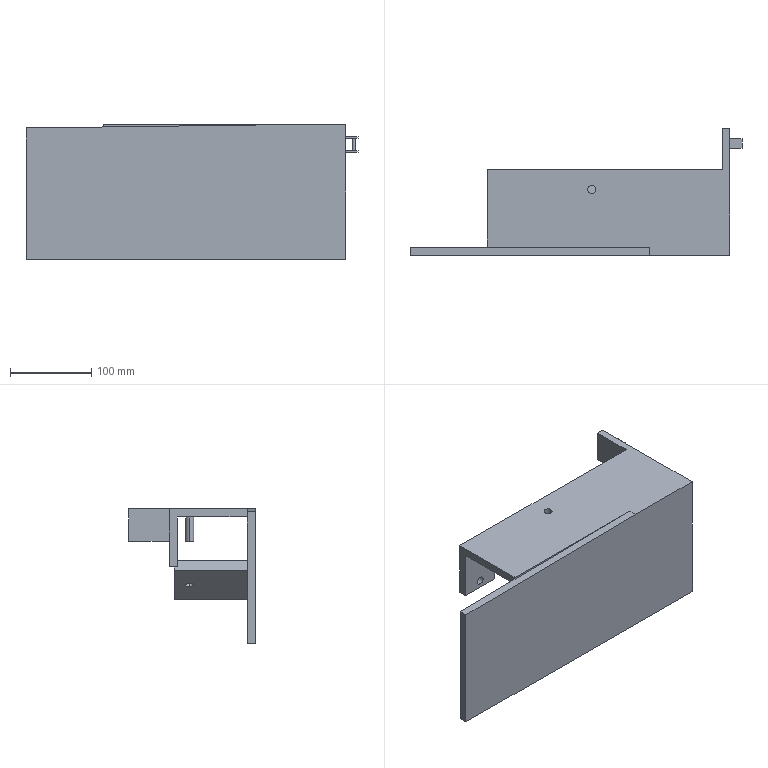Part | SolidWorks | features ICE 36, Extrusion 1, Sweep 1 | 1 solid | 46 faces | box 408.883 x 156 x 165.33 mm | volume 1077828 mm3 | plane 36 | cylinder 10 | commonest cylinder face diameters 10 x8 4 x2
STEP:
#1=CARTESIAN_POINT('',(-112.206,25.,-64.041));
#2=VERTEX_POINT('',#1);
#3=CARTESIAN_POINT('',(-121.034,25.,-59.342));
#4=VERTEX_POINT('',#3);
#5=CARTESIAN_POINT('',(-116.62,25.,-61.691));
#6=DIRECTION('',(-0.4698,0.,-0.8827));
#7=DIRECTION('',(-0.8827,0.,0.4698));
#8=AXIS2_PLACEMENT_3D('',#5,#6,#7);
#9=CIRCLE('',#8,5.);
#10=EDGE_CURVE('',#2,#4,#9,.T.);
#11=ORIENTED_EDGE('',*,*,#10,.F.);
#12=CARTESIAN_POINT('',(-118.59,25.,-76.034));
#13=VERTEX_POINT('',#12);
#14=CARTESIAN_POINT('',(-104.494,25.,-49.551));
#15=DIRECTION('',(-0.4698,0.,-0.8827));
#16=VECTOR('',#15,1000.);
#17=LINE('',#14,#16);
#18=EDGE_CURVE('',#2,#13,#17,.T.);
#19=ORIENTED_EDGE('',*,*,#18,.T.);
#20=CARTESIAN_POINT('',(-127.417,25.,-71.335));
#21=VERTEX_POINT('',#20);
#22=CARTESIAN_POINT('',(-123.003,25.,-73.685));
#23=DIRECTION('',(-0.4698,0.,-0.8827));
#24=DIRECTION('',(-0.8827,0.,0.4698));
#25=AXIS2_PLACEMENT_3D('',#22,#23,#24);
#26=CIRCLE('',#25,5.);
#27=EDGE_CURVE('',#13,#21,#26,.T.);
#28=ORIENTED_EDGE('',*,*,#27,.T.);
#29=CARTESIAN_POINT('',(-113.322,25.,-44.853));
#30=DIRECTION('',(-0.4698,0.,-0.8827));
#31=VECTOR('',#30,1000.);
#32=LINE('',#29,#31);
#33=EDGE_CURVE('',#4,#21,#32,.T.);
#34=ORIENTED_EDGE('',*,*,#33,.F.);
#35=EDGE_LOOP('',(#11,#19,#28,#34));
#36=FACE_OUTER_BOUND('',#35,.T.);
#37=CARTESIAN_POINT('',(-108.908,25.,-47.202));
#38=DIRECTION('',(-0.4698,0.,-0.8827));
#39=DIRECTION('',(-0.8827,0.,0.4698));
#40=AXIS2_PLACEMENT_3D('',#37,#38,#39);
#41=CYLINDRICAL_SURFACE('',#40,5.);
#42=ADVANCED_FACE('',(#36),#41,.F.);
#43=CARTESIAN_POINT('',(-209.637,40.,-45.397));
#44=VERTEX_POINT('',#43);
#45=CARTESIAN_POINT('',(-209.637,40.,-35.397));
#46=VERTEX_POINT('',#45);
#47=CARTESIAN_POINT('',(-209.637,40.,-40.397));
#48=DIRECTION('',(0.,1.,0.));
#49=DIRECTION('',(0.,0.,1.));
#50=AXIS2_PLACEMENT_3D('',#47,#48,#49);
#51=CIRCLE('',#50,5.);
#52=EDGE_CURVE('',#44,#46,#51,.T.);
#53=ORIENTED_EDGE('',*,*,#52,.F.);
#54=CARTESIAN_POINT('',(-209.637,50.,-45.397));
#55=VERTEX_POINT('',#54);
#56=CARTESIAN_POINT('',(-209.637,40.,-45.397));
#57=DIRECTION('',(0.,1.,0.));
#58=VECTOR('',#57,1000.);
#59=LINE('',#56,#58);
#60=EDGE_CURVE('',#44,#55,#59,.T.);
#61=ORIENTED_EDGE('',*,*,#60,.T.);
#62=CARTESIAN_POINT('',(-209.637,50.,-35.397));
#63=VERTEX_POINT('',#62);
#64=CARTESIAN_POINT('',(-209.637,50.,-40.397));
#65=DIRECTION('',(0.,1.,0.));
#66=DIRECTION('',(0.,0.,1.));
#67=AXIS2_PLACEMENT_3D('',#64,#65,#66);
#68=CIRCLE('',#67,5.);
#69=EDGE_CURVE('',#55,#63,#68,.T.);
#70=ORIENTED_EDGE('',*,*,#69,.T.);
#71=CARTESIAN_POINT('',(-209.637,40.,-35.397));
#72=DIRECTION('',(0.,1.,0.));
#73=VECTOR('',#72,1000.);
#74=LINE('',#71,#73);
#75=EDGE_CURVE('',#46,#63,#74,.T.);
#76=ORIENTED_EDGE('',*,*,#75,.F.);
#77=EDGE_LOOP('',(#53,#61,#70,#76));
#78=FACE_OUTER_BOUND('',#77,.T.);
#79=CARTESIAN_POINT('',(-209.637,40.,-40.397));
#80=DIRECTION('',(0.,1.,0.));
#81=DIRECTION('',(0.,0.,1.));
#82=AXIS2_PLACEMENT_3D('',#79,#80,#81);
#83=CYLINDRICAL_SURFACE('',#82,5.);
#84=ADVANCED_FACE('',(#78),#83,.F.);
#85=CARTESIAN_POINT('',(-101.44,25.,20.176));
#86=VERTEX_POINT('',#85);
#87=CARTESIAN_POINT('',(-111.44,25.,20.176));
#88=VERTEX_POINT('',#87);
#89=CARTESIAN_POINT('',(-106.44,25.,20.176));
#90=DIRECTION('',(0.,0.,-1.));
#91=DIRECTION('',(-1.,0.,0.));
#92=AXIS2_PLACEMENT_3D('',#89,#90,#91);
#93=CIRCLE('',#92,5.);
#94=EDGE_CURVE('',#86,#88,#93,.T.);
#95=ORIENTED_EDGE('',*,*,#94,.F.);
#96=CARTESIAN_POINT('',(-101.44,25.,10.176));
#97=VERTEX_POINT('',#96);
#98=CARTESIAN_POINT('',(-101.44,25.,210.176));
#99=DIRECTION('',(0.,0.,-1.));
#100=VECTOR('',#99,1000.);
#101=LINE('',#98,#100);
#102=EDGE_CURVE('',#86,#97,#101,.T.);
#103=ORIENTED_EDGE('',*,*,#102,.T.);
#104=CARTESIAN_POINT('',(-111.44,25.,10.176));
#105=VERTEX_POINT('',#104);
#106=CARTESIAN_POINT('',(-106.44,25.,10.176));
#107=DIRECTION('',(0.,0.,-1.));
#108=DIRECTION('',(-1.,0.,0.));
#109=AXIS2_PLACEMENT_3D('',#106,#107,#108);
#110=CIRCLE('',#109,5.);
#111=EDGE_CURVE('',#97,#105,#110,.T.);
#112=ORIENTED_EDGE('',*,*,#111,.T.);
#113=CARTESIAN_POINT('',(-111.44,25.,210.176));
#114=DIRECTION('',(0.,0.,-1.));
#115=VECTOR('',#114,1000.);
#116=LINE('',#113,#115);
#117=EDGE_CURVE('',#88,#105,#116,.T.);
#118=ORIENTED_EDGE('',*,*,#117,.F.);
#119=EDGE_LOOP('',(#95,#103,#112,#118));
#120=FACE_OUTER_BOUND('',#119,.T.);
#121=CARTESIAN_POINT('',(-106.44,25.,210.176));
#122=DIRECTION('',(0.,0.,-1.));
#123=DIRECTION('',(-1.,0.,0.));
#124=AXIS2_PLACEMENT_3D('',#121,#122,#123);
#125=CYLINDRICAL_SURFACE('',#124,5.);
#126=ADVANCED_FACE('',(#120),#125,.F.);
#127=CARTESIAN_POINT('',(71.457,81.541,-11.824));
#128=VERTEX_POINT('',#127);
#129=CARTESIAN_POINT('',(75.457,81.541,-11.824));
#130=VERTEX_POINT('',#129);
#131=CARTESIAN_POINT('',(73.457,81.541,-11.824));
#132=DIRECTION('',(0.,0.,-1.));
#133=DIRECTION('',(-1.,0.,0.));
#134=AXIS2_PLACEMENT_3D('',#131,#132,#133);
#135=CIRCLE('',#134,2.);
#136=EDGE_CURVE('',#128,#130,#135,.T.);
#137=ORIENTED_EDGE('',*,*,#136,.F.);
#138=CARTESIAN_POINT('',(71.457,81.541,3.56));
#139=VERTEX_POINT('',#138);
#140=CARTESIAN_POINT('',(71.457,81.541,-12.44));
#141=DIRECTION('',(0.,0.,1.));
#142=VECTOR('',#141,1000.);
#143=LINE('',#140,#142);
#144=EDGE_CURVE('',#128,#139,#143,.T.);
#145=ORIENTED_EDGE('',*,*,#144,.T.);
#146=CARTESIAN_POINT('',(75.457,81.541,3.56));
#147=VERTEX_POINT('',#146);
#148=CARTESIAN_POINT('',(73.457,81.541,3.56));
#149=DIRECTION('',(0.,0.,1.));
#150=DIRECTION('',(1.,0.,0.));
#151=AXIS2_PLACEMENT_3D('',#148,#149,#150);
#152=CIRCLE('',#151,2.);
#153=EDGE_CURVE('',#147,#139,#152,.T.);
#154=ORIENTED_EDGE('',*,*,#153,.F.);
#155=CARTESIAN_POINT('',(75.457,81.541,-12.44));
#156=DIRECTION('',(0.,0.,1.));
#157=VECTOR('',#156,1000.);
#158=LINE('',#155,#157);
#159=EDGE_CURVE('',#130,#147,#158,.T.);
#160=ORIENTED_EDGE('',*,*,#159,.F.);
#161=EDGE_LOOP('',(#137,#145,#154,#160));
#162=FACE_OUTER_BOUND('',#161,.T.);
#163=CARTESIAN_POINT('',(73.457,81.541,-12.44));
#164=DIRECTION('',(0.,0.,1.));
#165=DIRECTION('',(1.,0.,0.));
#166=AXIS2_PLACEMENT_3D('',#163,#164,#165);
#167=CYLINDRICAL_SURFACE('',#166,2.);
#168=ADVANCED_FACE('',(#162),#167,.T.);
#169=CARTESIAN_POINT('',(-21.44,25.,-19.824));
#170=VERTEX_POINT('',#169);
#171=CARTESIAN_POINT('',(-11.44,25.,-19.824));
#172=VERTEX_POINT('',#171);
#173=CARTESIAN_POINT('',(-16.44,25.,-19.824));
#174=DIRECTION('',(0.,0.,-1.));
#175=DIRECTION('',(1.,0.,0.));
#176=AXIS2_PLACEMENT_3D('',#173,#174,#175);
#177=CIRCLE('',#176,5.);
#178=EDGE_CURVE('',#170,#172,#177,.T.);
#179=ORIENTED_EDGE('',*,*,#178,.F.);
#180=CARTESIAN_POINT('',(-21.44,25.,10.176));
#181=VERTEX_POINT('',#180);
#182=CARTESIAN_POINT('',(-21.44,25.,-33.966));
#183=DIRECTION('',(0.,0.,1.));
#184=VECTOR('',#183,1000.);
#185=LINE('',#182,#184);
#186=EDGE_CURVE('',#170,#181,#185,.T.);
#187=ORIENTED_EDGE('',*,*,#186,.T.);
#188=CARTESIAN_POINT('',(-11.44,25.,10.176));
#189=VERTEX_POINT('',#188);
#190=CARTESIAN_POINT('',(-16.44,25.,10.176));
#191=DIRECTION('',(0.,0.,-1.));
#192=DIRECTION('',(1.,0.,0.));
#193=AXIS2_PLACEMENT_3D('',#190,#191,#192);
#194=CIRCLE('',#193,5.);
#195=EDGE_CURVE('',#181,#189,#194,.T.);
#196=ORIENTED_EDGE('',*,*,#195,.T.);
#197=CARTESIAN_POINT('',(-11.44,25.,-33.966));
#198=DIRECTION('',(0.,0.,1.));
#199=VECTOR('',#198,1000.);
#200=LINE('',#197,#199);
#201=EDGE_CURVE('',#172,#189,#200,.T.);
#202=ORIENTED_EDGE('',*,*,#201,.F.);
#203=EDGE_LOOP('',(#179,#187,#196,#202));
#204=FACE_OUTER_BOUND('',#203,.T.);
#205=CARTESIAN_POINT('',(-16.44,25.,-33.966));
#206=DIRECTION('',(0.,0.,1.));
#207=DIRECTION('',(1.,0.,0.));
#208=AXIS2_PLACEMENT_3D('',#205,#206,#207);
#209=CYLINDRICAL_SURFACE('',#208,5.);
#210=ADVANCED_FACE('',(#204),#209,.T.);
#211=CARTESIAN_POINT('',(63.457,-46.,10.176));
#212=VERTEX_POINT('',#211);
#213=CARTESIAN_POINT('',(63.457,-46.,-145.154));
#214=VERTEX_POINT('',#213);
#215=CARTESIAN_POINT('',(63.457,-46.,20.176));
#216=DIRECTION('',(0.,0.,-1.));
#217=VECTOR('',#216,1000.);
#218=LINE('',#215,#217);
#219=EDGE_CURVE('',#212,#214,#218,.T.);
#220=ORIENTED_EDGE('',*,*,#219,.T.);
#221=CARTESIAN_POINT('',(-330.425,-46.,-145.154));
#222=VERTEX_POINT('',#221);
#223=CARTESIAN_POINT('',(-330.425,-46.,-145.154));
#224=DIRECTION('',(1.,0.,0.));
#225=VECTOR('',#224,1000.);
#226=LINE('',#223,#225);
#227=EDGE_CURVE('',#222,#214,#226,.T.);
#228=ORIENTED_EDGE('',*,*,#227,.F.);
#229=CARTESIAN_POINT('',(-330.425,-46.,16.345));
#230=VERTEX_POINT('',#229);
#231=CARTESIAN_POINT('',(-330.425,-46.,-189.172));
#232=DIRECTION('',(0.,0.,-1.));
#233=VECTOR('',#232,1000.);
#234=LINE('',#231,#233);
#235=EDGE_CURVE('',#230,#222,#234,.T.);
#236=ORIENTED_EDGE('',*,*,#235,.F.);
#237=CARTESIAN_POINT('',(-235.023,-46.,17.582));
#238=VERTEX_POINT('',#237);
#239=CARTESIAN_POINT('',(-35.023,-46.,20.176));
#240=DIRECTION('',(0.9999,0.,0.01297));
#241=VECTOR('',#240,1000.);
#242=LINE('',#239,#241);
#243=EDGE_CURVE('',#230,#238,#242,.T.);
#244=ORIENTED_EDGE('',*,*,#243,.T.);
#245=CARTESIAN_POINT('',(-235.023,-46.,10.176));
#246=VERTEX_POINT('',#245);
#247=CARTESIAN_POINT('',(-235.023,-46.,10.176));
#248=DIRECTION('',(0.,0.,1.));
#249=VECTOR('',#248,1000.);
#250=LINE('',#247,#249);
#251=EDGE_CURVE('',#246,#238,#250,.T.);
#252=ORIENTED_EDGE('',*,*,#251,.F.);
#253=CARTESIAN_POINT('',(-35.023,-46.,10.176));
#254=DIRECTION('',(-1.,0.,0.));
#255=VECTOR('',#254,1000.);
#256=LINE('',#253,#255);
#257=EDGE_CURVE('',#212,#246,#256,.T.);
#258=ORIENTED_EDGE('',*,*,#257,.F.);
#259=EDGE_LOOP('',(#220,#228,#236,#244,#252,#258));
#260=FACE_OUTER_BOUND('',#259,.T.);
#261=CARTESIAN_POINT('',(-88.62,-46.,-91.985));
#262=VERTEX_POINT('',#261);
#263=CARTESIAN_POINT('',(-157.387,-46.,-55.384));
#264=VERTEX_POINT('',#263);
#265=CARTESIAN_POINT('',(-100.648,-46.,-85.583));
#266=DIRECTION('',(-0.8827,0.,0.4698));
#267=VECTOR('',#266,1000.);
#268=LINE('',#265,#267);
#269=EDGE_CURVE('',#262,#264,#268,.T.);
#270=ORIENTED_EDGE('',*,*,#269,.F.);
#271=CARTESIAN_POINT('',(-82.236,-46.,-79.992));
#272=VERTEX_POINT('',#271);
#273=CARTESIAN_POINT('',(-88.62,-46.,-91.985));
#274=DIRECTION('',(-0.4698,0.,-0.8827));
#275=VECTOR('',#274,1000.);
#276=LINE('',#273,#275);
#277=EDGE_CURVE('',#272,#262,#276,.T.);
#278=ORIENTED_EDGE('',*,*,#277,.F.);
#279=CARTESIAN_POINT('',(-151.003,-46.,-43.391));
#280=VERTEX_POINT('',#279);
#281=CARTESIAN_POINT('',(-82.236,-46.,-79.992));
#282=DIRECTION('',(0.8827,0.,-0.4698));
#283=VECTOR('',#282,1000.);
#284=LINE('',#281,#283);
#285=EDGE_CURVE('',#280,#272,#284,.T.);
#286=ORIENTED_EDGE('',*,*,#285,.F.);
#287=CARTESIAN_POINT('',(-157.387,-46.,-55.384));
#288=DIRECTION('',(0.4698,0.,0.8827));
#289=VECTOR('',#288,1000.);
#290=LINE('',#287,#289);
#291=EDGE_CURVE('',#264,#280,#290,.T.);
#292=ORIENTED_EDGE('',*,*,#291,.F.);
#293=EDGE_LOOP('',(#270,#278,#286,#292));
#294=FACE_BOUND('',#293,.T.);
#295=CARTESIAN_POINT('',(0.,-46.,0.));
#296=DIRECTION('',(0.,-1.,0.));
#297=DIRECTION('',(0.,0.,-1.));
#298=AXIS2_PLACEMENT_3D('',#295,#296,#297);
#299=PLANE('',#298);
#300=ADVANCED_FACE('',(#260,#294),#299,.F.);
#301=CARTESIAN_POINT('',(-209.637,50.,-40.397));
#302=DIRECTION('',(0.,1.,0.));
#303=DIRECTION('',(0.,0.,1.));
#304=AXIS2_PLACEMENT_3D('',#301,#302,#303);
#305=CIRCLE('',#304,5.);
#306=EDGE_CURVE('',#63,#55,#305,.T.);
#307=ORIENTED_EDGE('',*,*,#306,.F.);
#308=ORIENTED_EDGE('',*,*,#69,.F.);
#309=EDGE_LOOP('',(#307,#308));
#310=FACE_BOUND('',#309,.T.);
#311=CARTESIAN_POINT('',(-184.251,50.,10.176));
#312=VERTEX_POINT('',#311);
#313=CARTESIAN_POINT('',(54.56,50.,10.176));
#314=VERTEX_POINT('',#313);
#315=CARTESIAN_POINT('',(-161.43,50.,10.176));
#316=DIRECTION('',(1.,0.,0.));
#317=VECTOR('',#316,1000.);
#318=LINE('',#315,#317);
#319=EDGE_CURVE('',#312,#314,#318,.T.);
#320=ORIENTED_EDGE('',*,*,#319,.F.);
#321=CARTESIAN_POINT('',(-184.251,50.,-50.397));
#322=VERTEX_POINT('',#321);
#323=CARTESIAN_POINT('',(-184.251,50.,10.176));
#324=DIRECTION('',(0.,0.,-1.));
#325=VECTOR('',#324,1000.);
#326=LINE('',#323,#325);
#327=EDGE_CURVE('',#312,#322,#326,.T.);
#328=ORIENTED_EDGE('',*,*,#327,.T.);
#329=CARTESIAN_POINT('',(-235.023,50.,-50.397));
#330=VERTEX_POINT('',#329);
#331=CARTESIAN_POINT('',(-235.023,50.,-50.397));
#332=DIRECTION('',(-1.,0.,0.));
#333=VECTOR('',#332,1000.);
#334=LINE('',#331,#333);
#335=EDGE_CURVE('',#322,#330,#334,.T.);
#336=ORIENTED_EDGE('',*,*,#335,.T.);
#337=CARTESIAN_POINT('',(-235.023,50.,20.176));
#338=VERTEX_POINT('',#337);
#339=CARTESIAN_POINT('',(-235.023,50.,10.176));
#340=DIRECTION('',(0.,0.,-1.));
#341=VECTOR('',#340,1000.);
#342=LINE('',#339,#341);
#343=EDGE_CURVE('',#338,#330,#342,.T.);
#344=ORIENTED_EDGE('',*,*,#343,.F.);
#345=CARTESIAN_POINT('',(54.56,50.,20.176));
#346=VERTEX_POINT('',#345);
#347=CARTESIAN_POINT('',(-110.44,50.,20.176));
#348=DIRECTION('',(-1.,0.,0.));
#349=VECTOR('',#348,1000.);
#350=LINE('',#347,#349);
#351=EDGE_CURVE('',#346,#338,#350,.T.);
#352=ORIENTED_EDGE('',*,*,#351,.F.);
#353=CARTESIAN_POINT('',(54.56,50.,20.176));
#354=DIRECTION('',(0.,0.,-1.));
#355=VECTOR('',#354,1000.);
#356=LINE('',#353,#355);
#357=EDGE_CURVE('',#346,#314,#356,.T.);
#358=ORIENTED_EDGE('',*,*,#357,.T.);
#359=EDGE_LOOP('',(#320,#328,#336,#344,#352,#358));
#360=FACE_OUTER_BOUND('',#359,.T.);
#361=CARTESIAN_POINT('',(0.,50.,0.));
#362=DIRECTION('',(0.,-1.,0.));
#363=DIRECTION('',(0.,0.,-1.));
#364=AXIS2_PLACEMENT_3D('',#361,#362,#363);
#365=PLANE('',#364);
#366=ADVANCED_FACE('',(#310,#360),#365,.F.);
#367=CARTESIAN_POINT('',(-106.44,25.,20.176));
#368=DIRECTION('',(0.,0.,-1.));
#369=DIRECTION('',(-1.,0.,0.));
#370=AXIS2_PLACEMENT_3D('',#367,#368,#369);
#371=CIRCLE('',#370,5.);
#372=EDGE_CURVE('',#88,#86,#371,.T.);
#373=ORIENTED_EDGE('',*,*,#372,.T.);
#374=ORIENTED_EDGE('',*,*,#94,.T.);
#375=EDGE_LOOP('',(#373,#374));
#376=FACE_BOUND('',#375,.T.);
#377=ORIENTED_EDGE('',*,*,#351,.T.);
#378=CARTESIAN_POINT('',(-235.023,-46.,20.176));
#379=VERTEX_POINT('',#378);
#380=CARTESIAN_POINT('',(-235.023,50.,20.176));
#381=DIRECTION('',(0.,1.,0.));
#382=VECTOR('',#381,1000.);
#383=LINE('',#380,#382);
#384=EDGE_CURVE('',#379,#338,#383,.T.);
#385=ORIENTED_EDGE('',*,*,#384,.F.);
#386=CARTESIAN_POINT('',(-35.023,-46.,20.176));
#387=VERTEX_POINT('',#386);
#388=CARTESIAN_POINT('',(-235.023,-46.,20.176));
#389=DIRECTION('',(1.,0.,0.));
#390=VECTOR('',#389,1000.);
#391=LINE('',#388,#390);
#392=EDGE_CURVE('',#379,#387,#391,.T.);
#393=ORIENTED_EDGE('',*,*,#392,.T.);
#394=CARTESIAN_POINT('',(-35.023,-56.,20.176));
#395=VERTEX_POINT('',#394);
#396=CARTESIAN_POINT('',(-35.023,-46.,20.176));
#397=DIRECTION('',(0.,-1.,0.));
#398=VECTOR('',#397,1000.);
#399=LINE('',#396,#398);
#400=EDGE_CURVE('',#387,#395,#399,.T.);
#401=ORIENTED_EDGE('',*,*,#400,.T.);
#402=CARTESIAN_POINT('',(63.457,-56.,20.176));
#403=VERTEX_POINT('',#402);
#404=CARTESIAN_POINT('',(-35.023,-56.,20.176));
#405=DIRECTION('',(1.,0.,0.));
#406=VECTOR('',#405,1000.);
#407=LINE('',#404,#406);
#408=EDGE_CURVE('',#395,#403,#407,.T.);
#409=ORIENTED_EDGE('',*,*,#408,.T.);
#410=CARTESIAN_POINT('',(63.457,100.,20.176));
#411=VERTEX_POINT('',#410);
#412=CARTESIAN_POINT('',(63.457,-0.000025,20.176));
#413=DIRECTION('',(0.,1.,0.));
#414=VECTOR('',#413,1000.);
#415=LINE('',#412,#414);
#416=EDGE_CURVE('',#403,#411,#415,.T.);
#417=ORIENTED_EDGE('',*,*,#416,.T.);
#418=CARTESIAN_POINT('',(54.56,100.,20.176));
#419=VERTEX_POINT('',#418);
#420=CARTESIAN_POINT('',(54.56,100.,20.176));
#421=DIRECTION('',(-1.,0.,0.));
#422=VECTOR('',#421,1000.);
#423=LINE('',#420,#422);
#424=EDGE_CURVE('',#411,#419,#423,.T.);
#425=ORIENTED_EDGE('',*,*,#424,.T.);
#426=CARTESIAN_POINT('',(54.56,100.,20.176));
#427=DIRECTION('',(0.,-1.,0.));
#428=VECTOR('',#427,1000.);
#429=LINE('',#426,#428);
#430=EDGE_CURVE('',#419,#346,#429,.T.);
#431=ORIENTED_EDGE('',*,*,#430,.T.);
#432=EDGE_LOOP('',(#377,#385,#393,#401,#409,#417,#425,#431));
#433=FACE_OUTER_BOUND('',#432,.T.);
#434=CARTESIAN_POINT('',(0.,0.,20.176));
#435=DIRECTION('',(0.,0.,-1.));
#436=DIRECTION('',(-1.,0.,0.));
#437=AXIS2_PLACEMENT_3D('',#434,#435,#436);
#438=PLANE('',#437);
#439=ADVANCED_FACE('',(#376,#433),#438,.F.);
#440=CARTESIAN_POINT('',(-106.44,25.,10.176));
#441=DIRECTION('',(0.,0.,-1.));
#442=DIRECTION('',(-1.,0.,0.));
#443=AXIS2_PLACEMENT_3D('',#440,#441,#442);
#444=CIRCLE('',#443,5.);
#445=EDGE_CURVE('',#105,#97,#444,.T.);
#446=ORIENTED_EDGE('',*,*,#445,.F.);
#447=ORIENTED_EDGE('',*,*,#111,.F.);
#448=EDGE_LOOP('',(#446,#447));
#449=FACE_BOUND('',#448,.T.);
#450=CARTESIAN_POINT('',(-16.44,25.,10.176));
#451=DIRECTION('',(0.,0.,-1.));
#452=DIRECTION('',(1.,0.,0.));
#453=AXIS2_PLACEMENT_3D('',#450,#451,#452);
#454=CIRCLE('',#453,5.);
#455=EDGE_CURVE('',#189,#181,#454,.T.);
#456=ORIENTED_EDGE('',*,*,#455,.F.);
#457=ORIENTED_EDGE('',*,*,#195,.F.);
#458=EDGE_LOOP('',(#456,#457));
#459=FACE_BOUND('',#458,.T.);
#460=CARTESIAN_POINT('',(-235.023,40.,10.176));
#461=VERTEX_POINT('',#460);
#462=CARTESIAN_POINT('',(-184.251,40.,10.176));
#463=VERTEX_POINT('',#462);
#464=CARTESIAN_POINT('',(-235.023,40.,10.176));
#465=DIRECTION('',(1.,0.,0.));
#466=VECTOR('',#465,1000.);
#467=LINE('',#464,#466);
#468=EDGE_CURVE('',#461,#463,#467,.T.);
#469=ORIENTED_EDGE('',*,*,#468,.T.);
#470=CARTESIAN_POINT('',(-184.251,40.,10.176));
#471=DIRECTION('',(0.,1.,0.));
#472=VECTOR('',#471,1000.);
#473=LINE('',#470,#472);
#474=EDGE_CURVE('',#463,#312,#473,.T.);
#475=ORIENTED_EDGE('',*,*,#474,.T.);
#476=ORIENTED_EDGE('',*,*,#319,.T.);
#477=CARTESIAN_POINT('',(54.56,45.,10.176));
#478=VERTEX_POINT('',#477);
#479=CARTESIAN_POINT('',(54.56,100.,10.176));
#480=DIRECTION('',(0.,1.,0.));
#481=VECTOR('',#480,1000.);
#482=LINE('',#479,#481);
#483=EDGE_CURVE('',#478,#314,#482,.T.);
#484=ORIENTED_EDGE('',*,*,#483,.F.);
#485=CARTESIAN_POINT('',(63.457,45.,10.176));
#486=VERTEX_POINT('',#485);
#487=CARTESIAN_POINT('',(-161.43,45.,10.176));
#488=DIRECTION('',(-1.,0.,0.));
#489=VECTOR('',#488,1000.);
#490=LINE('',#487,#489);
#491=EDGE_CURVE('',#486,#478,#490,.T.);
#492=ORIENTED_EDGE('',*,*,#491,.F.);
#493=CARTESIAN_POINT('',(63.457,0.,10.176));
#494=DIRECTION('',(0.,-1.,0.));
#495=VECTOR('',#494,1000.);
#496=LINE('',#493,#495);
#497=EDGE_CURVE('',#486,#212,#496,.T.);
#498=ORIENTED_EDGE('',*,*,#497,.T.);
#499=ORIENTED_EDGE('',*,*,#257,.T.);
#500=CARTESIAN_POINT('',(-235.023,50.,10.176));
#501=DIRECTION('',(0.,-1.,0.));
#502=VECTOR('',#501,1000.);
#503=LINE('',#500,#502);
#504=EDGE_CURVE('',#461,#246,#503,.T.);
#505=ORIENTED_EDGE('',*,*,#504,.F.);
#506=EDGE_LOOP('',(#469,#475,#476,#484,#492,#498,#499,#505));
#507=FACE_OUTER_BOUND('',#506,.T.);
#508=CARTESIAN_POINT('',(-161.43,0.,10.176));
#509=DIRECTION('',(0.,0.,1.));
#510=DIRECTION('',(1.,0.,0.));
#511=AXIS2_PLACEMENT_3D('',#508,#509,#510);
#512=PLANE('',#511);
#513=ADVANCED_FACE('',(#449,#459,#507),#512,.F.);
#514=CARTESIAN_POINT('',(63.457,-56.,-145.154));
#515=VERTEX_POINT('',#514);
#516=CARTESIAN_POINT('',(63.457,-56.,20.176));
#517=DIRECTION('',(0.,0.,-1.));
#518=VECTOR('',#517,1000.);
#519=LINE('',#516,#518);
#520=EDGE_CURVE('',#403,#515,#519,.T.);
#521=ORIENTED_EDGE('',*,*,#520,.T.);
#522=CARTESIAN_POINT('',(63.457,-76.,-145.154));
#523=DIRECTION('',(0.,1.,0.));
#524=VECTOR('',#523,1000.);
#525=LINE('',#522,#524);
#526=EDGE_CURVE('',#515,#214,#525,.T.);
#527=ORIENTED_EDGE('',*,*,#526,.T.);
#528=ORIENTED_EDGE('',*,*,#219,.F.);
#529=ORIENTED_EDGE('',*,*,#497,.F.);
#530=CARTESIAN_POINT('',(63.457,45.,-19.824));
#531=VERTEX_POINT('',#530);
#532=CARTESIAN_POINT('',(63.457,45.,0.));
#533=DIRECTION('',(0.,0.,1.));
#534=VECTOR('',#533,1000.);
#535=LINE('',#532,#534);
#536=EDGE_CURVE('',#531,#486,#535,.T.);
#537=ORIENTED_EDGE('',*,*,#536,.F.);
#538=CARTESIAN_POINT('',(63.457,50.,-19.824));
#539=VERTEX_POINT('',#538);
#540=CARTESIAN_POINT('',(63.457,100.001,-19.824));
#541=DIRECTION('',(0.,-1.,0.));
#542=VECTOR('',#541,1000.);
#543=LINE('',#540,#542);
#544=EDGE_CURVE('',#539,#531,#543,.T.);
#545=ORIENTED_EDGE('',*,*,#544,.F.);
#546=CARTESIAN_POINT('',(63.457,50.,-19.755));
#547=VERTEX_POINT('',#546);
#548=CARTESIAN_POINT('',(63.457,50.,20.176));
#549=DIRECTION('',(0.,0.,1.));
#550=VECTOR('',#549,1000.);
#551=LINE('',#548,#550);
#552=EDGE_CURVE('',#539,#547,#551,.T.);
#553=ORIENTED_EDGE('',*,*,#552,.T.);
#554=CARTESIAN_POINT('',(63.457,100.,-19.755));
#555=VERTEX_POINT('',#554);
#556=CARTESIAN_POINT('',(63.457,100.,-19.755));
#557=DIRECTION('',(0.,-1.,0.));
#558=VECTOR('',#557,1000.);
#559=LINE('',#556,#558);
#560=EDGE_CURVE('',#555,#547,#559,.T.);
#561=ORIENTED_EDGE('',*,*,#560,.F.);
#562=CARTESIAN_POINT('',(63.457,100.,10.176));
#563=DIRECTION('',(0.,0.,-1.));
#564=VECTOR('',#563,1000.);
#565=LINE('',#562,#564);
#566=EDGE_CURVE('',#411,#555,#565,.T.);
#567=ORIENTED_EDGE('',*,*,#566,.F.);
#568=ORIENTED_EDGE('',*,*,#416,.F.);
#569=EDGE_LOOP('',(#521,#527,#528,#529,#537,#545,#553,#561,#567,#568));
#570=FACE_OUTER_BOUND('',#569,.T.);
#571=CARTESIAN_POINT('',(63.457,87.541,-11.824));
#572=VERTEX_POINT('',#571);
#573=CARTESIAN_POINT('',(63.457,75.541,-11.824));
#574=VERTEX_POINT('',#573);
#575=CARTESIAN_POINT('',(63.457,75.541,-11.824));
#576=DIRECTION('',(0.,-1.,0.));
#577=VECTOR('',#576,1000.);
#578=LINE('',#575,#577);
#579=EDGE_CURVE('',#572,#574,#578,.T.);
#580=ORIENTED_EDGE('',*,*,#579,.F.);
#581=CARTESIAN_POINT('',(63.457,87.541,-13.824));
#582=VERTEX_POINT('',#581);
#583=CARTESIAN_POINT('',(63.457,87.541,-11.824));
#584=DIRECTION('',(0.,0.,1.));
#585=VECTOR('',#584,1000.);
#586=LINE('',#583,#585);
#587=EDGE_CURVE('',#582,#572,#586,.T.);
#588=ORIENTED_EDGE('',*,*,#587,.F.);
#589=CARTESIAN_POINT('',(63.457,75.541,-13.824));
#590=VERTEX_POINT('',#589);
#591=CARTESIAN_POINT('',(63.457,87.541,-13.824));
#592=DIRECTION('',(0.,1.,0.));
#593=VECTOR('',#592,1000.);
#594=LINE('',#591,#593);
#595=EDGE_CURVE('',#590,#582,#594,.T.);
#596=ORIENTED_EDGE('',*,*,#595,.F.);
#597=CARTESIAN_POINT('',(63.457,75.541,-13.824));
#598=DIRECTION('',(0.,0.,-1.));
#599=VECTOR('',#598,1000.);
#600=LINE('',#597,#599);
#601=EDGE_CURVE('',#574,#590,#600,.T.);
#602=ORIENTED_EDGE('',*,*,#601,.F.);
#603=EDGE_LOOP('',(#580,#588,#596,#602));
#604=FACE_BOUND('',#603,.T.);
#605=CARTESIAN_POINT('',(63.457,75.541,5.56));
#606=VERTEX_POINT('',#605);
#607=CARTESIAN_POINT('',(63.457,75.541,3.56));
#608=VERTEX_POINT('',#607);
#609=CARTESIAN_POINT('',(63.457,75.541,3.56));
#610=DIRECTION('',(0.,0.,-1.));
#611=VECTOR('',#610,1000.);
#612=LINE('',#609,#611);
#613=EDGE_CURVE('',#606,#608,#612,.T.);
#614=ORIENTED_EDGE('',*,*,#613,.F.);
#615=CARTESIAN_POINT('',(63.457,87.541,5.56));
#616=VERTEX_POINT('',#615);
#617=CARTESIAN_POINT('',(63.457,87.541,5.56));
#618=DIRECTION('',(0.,-1.,0.));
#619=VECTOR('',#618,1000.);
#620=LINE('',#617,#619);
#621=EDGE_CURVE('',#616,#606,#620,.T.);
#622=ORIENTED_EDGE('',*,*,#621,.F.);
#623=CARTESIAN_POINT('',(63.457,87.541,3.56));
#624=VERTEX_POINT('',#623);
#625=CARTESIAN_POINT('',(63.457,87.541,3.56));
#626=DIRECTION('',(0.,0.,1.));
#627=VECTOR('',#626,1000.);
#628=LINE('',#625,#627);
#629=EDGE_CURVE('',#624,#616,#628,.T.);
#630=ORIENTED_EDGE('',*,*,#629,.F.);
#631=CARTESIAN_POINT('',(63.457,87.541,3.56));
#632=DIRECTION('',(0.,1.,0.));
#633=VECTOR('',#632,1000.);
#634=LINE('',#631,#633);
#635=EDGE_CURVE('',#608,#624,#634,.T.);
#636=ORIENTED_EDGE('',*,*,#635,.F.);
#637=EDGE_LOOP('',(#614,#622,#630,#636));
#638=FACE_BOUND('',#637,.T.);
#639=CARTESIAN_POINT('',(63.457,-0.000025,20.176));
#640=DIRECTION('',(-1.,0.,0.));
#641=DIRECTION('',(0.,0.,1.));
#642=AXIS2_PLACEMENT_3D('',#639,#640,#641);
#643=PLANE('',#642);
#644=ADVANCED_FACE('',(#570,#604,#638),#643,.F.);
#645=CARTESIAN_POINT('',(54.56,50.,-19.824));
#646=VERTEX_POINT('',#645);
#647=CARTESIAN_POINT('',(-110.44,50.,-19.824));
#648=DIRECTION('',(-1.,0.,0.));
#649=VECTOR('',#648,1000.);
#650=LINE('',#647,#649);
#651=EDGE_CURVE('',#539,#646,#650,.T.);
#652=ORIENTED_EDGE('',*,*,#651,.T.);
#653=CARTESIAN_POINT('',(54.56,50.,-19.755));
#654=VERTEX_POINT('',#653);
#655=CARTESIAN_POINT('',(54.56,50.,0.));
#656=DIRECTION('',(0.,0.,1.));
#657=VECTOR('',#656,1000.);
#658=LINE('',#655,#657);
#659=EDGE_CURVE('',#646,#654,#658,.T.);
#660=ORIENTED_EDGE('',*,*,#659,.T.);
#661=CARTESIAN_POINT('',(46.523,50.,-19.755));
#662=DIRECTION('',(-1.,0.,0.));
#663=VECTOR('',#662,1000.);
#664=LINE('',#661,#663);
#665=EDGE_CURVE('',#547,#654,#664,.T.);
#666=ORIENTED_EDGE('',*,*,#665,.F.);
#667=ORIENTED_EDGE('',*,*,#552,.F.);
#668=EDGE_LOOP('',(#652,#660,#666,#667));
#669=FACE_OUTER_BOUND('',#668,.T.);
#670=CARTESIAN_POINT('',(0.,50.,0.));
#671=DIRECTION('',(0.,-1.,0.));
#672=DIRECTION('',(0.,0.,-1.));
#673=AXIS2_PLACEMENT_3D('',#670,#671,#672);
#674=PLANE('',#673);
#675=ADVANCED_FACE('',(#669),#674,.F.);
#676=ORIENTED_EDGE('',*,*,#186,.F.);
#677=CARTESIAN_POINT('',(-16.44,25.,-19.824));
#678=DIRECTION('',(0.,0.,-1.));
#679=DIRECTION('',(1.,0.,0.));
#680=AXIS2_PLACEMENT_3D('',#677,#678,#679);
#681=CIRCLE('',#680,5.);
#682=EDGE_CURVE('',#172,#170,#681,.T.);
#683=ORIENTED_EDGE('',*,*,#682,.F.);
#684=ORIENTED_EDGE('',*,*,#201,.T.);
#685=ORIENTED_EDGE('',*,*,#455,.T.);
#686=EDGE_LOOP('',(#676,#683,#684,#685));
#687=FACE_OUTER_BOUND('',#686,.T.);
#688=CARTESIAN_POINT('',(-16.44,25.,-33.966));
#689=DIRECTION('',(0.,0.,1.));
#690=DIRECTION('',(1.,0.,0.));
#691=AXIS2_PLACEMENT_3D('',#688,#689,#690);
#692=CYLINDRICAL_SURFACE('',#691,5.);
#693=ADVANCED_FACE('',(#687),#692,.T.);
#694=CARTESIAN_POINT('',(54.56,45.,-19.824));
#695=VERTEX_POINT('',#694);
#696=CARTESIAN_POINT('',(54.56,45.,2.176));
#697=DIRECTION('',(0.,0.,1.));
#698=VECTOR('',#697,1000.);
#699=LINE('',#696,#698);
#700=EDGE_CURVE('',#695,#478,#699,.T.);
#701=ORIENTED_EDGE('',*,*,#700,.T.);
#702=ORIENTED_EDGE('',*,*,#483,.T.);
#703=ORIENTED_EDGE('',*,*,#357,.F.);
#704=ORIENTED_EDGE('',*,*,#430,.F.);
#705=CARTESIAN_POINT('',(54.56,100.,-19.755));
#706=VERTEX_POINT('',#705);
#707=CARTESIAN_POINT('',(54.56,100.,2.176));
#708=DIRECTION('',(0.,0.,1.));
#709=VECTOR('',#708,1000.);
#710=LINE('',#707,#709);
#711=EDGE_CURVE('',#706,#419,#710,.T.);
#712=ORIENTED_EDGE('',*,*,#711,.F.);
#713=CARTESIAN_POINT('',(54.56,100.,-19.755));
#714=DIRECTION('',(0.,1.,0.));
#715=VECTOR('',#714,1000.);
#716=LINE('',#713,#715);
#717=EDGE_CURVE('',#654,#706,#716,.T.);
#718=ORIENTED_EDGE('',*,*,#717,.F.);
#719=ORIENTED_EDGE('',*,*,#659,.F.);
#720=CARTESIAN_POINT('',(54.56,100.001,-19.824));
#721=DIRECTION('',(0.,1.,0.));
#722=VECTOR('',#721,1000.);
#723=LINE('',#720,#722);
#724=EDGE_CURVE('',#695,#646,#723,.T.);
#725=ORIENTED_EDGE('',*,*,#724,.F.);
#726=EDGE_LOOP('',(#701,#702,#703,#704,#712,#718,#719,#725));
#727=FACE_OUTER_BOUND('',#726,.T.);
#728=CARTESIAN_POINT('',(54.56,45.,2.176));
#729=DIRECTION('',(-1.,0.,0.));
#730=DIRECTION('',(0.,0.,1.));
#731=AXIS2_PLACEMENT_3D('',#728,#729,#730);
#732=PLANE('',#731);
#733=ADVANCED_FACE('',(#727),#732,.T.);
#734=ORIENTED_EDGE('',*,*,#491,.T.);
#735=ORIENTED_EDGE('',*,*,#700,.F.);
#736=CARTESIAN_POINT('',(-110.44,45.,-19.824));
#737=DIRECTION('',(-1.,0.,0.));
#738=VECTOR('',#737,1000.);
#739=LINE('',#736,#738);
#740=EDGE_CURVE('',#531,#695,#739,.T.);
#741=ORIENTED_EDGE('',*,*,#740,.F.);
#742=ORIENTED_EDGE('',*,*,#536,.T.);
#743=EDGE_LOOP('',(#734,#735,#741,#742));
#744=FACE_OUTER_BOUND('',#743,.T.);
#745=CARTESIAN_POINT('',(0.,45.,0.));
#746=DIRECTION('',(0.,1.,0.));
#747=DIRECTION('',(0.,0.,1.));
#748=AXIS2_PLACEMENT_3D('',#745,#746,#747);
#749=PLANE('',#748);
#750=ADVANCED_FACE('',(#744),#749,.F.);
#751=ORIENTED_EDGE('',*,*,#665,.T.);
#752=ORIENTED_EDGE('',*,*,#717,.T.);
#753=CARTESIAN_POINT('',(46.523,100.,-19.755));
#754=DIRECTION('',(-1.,0.,0.));
#755=VECTOR('',#754,1000.);
#756=LINE('',#753,#755);
#757=EDGE_CURVE('',#555,#706,#756,.T.);
#758=ORIENTED_EDGE('',*,*,#757,.F.);
#759=ORIENTED_EDGE('',*,*,#560,.T.);
#760=EDGE_LOOP('',(#751,#752,#758,#759));
#761=FACE_OUTER_BOUND('',#760,.T.);
#762=CARTESIAN_POINT('',(46.523,100.,-19.755));
#763=DIRECTION('',(0.,0.,1.));
#764=DIRECTION('',(1.,0.,0.));
#765=AXIS2_PLACEMENT_3D('',#762,#763,#764);
#766=PLANE('',#765);
#767=ADVANCED_FACE('',(#761),#766,.F.);
#768=ORIENTED_EDGE('',*,*,#711,.T.);
#769=ORIENTED_EDGE('',*,*,#424,.F.);
#770=ORIENTED_EDGE('',*,*,#566,.T.);
#771=ORIENTED_EDGE('',*,*,#757,.T.);
#772=EDGE_LOOP('',(#768,#769,#770,#771));
#773=FACE_OUTER_BOUND('',#772,.T.);
#774=CARTESIAN_POINT('',(0.,100.,0.));
#775=DIRECTION('',(0.,1.,0.));
#776=DIRECTION('',(0.,0.,1.));
#777=AXIS2_PLACEMENT_3D('',#774,#775,#776);
#778=PLANE('',#777);
#779=ADVANCED_FACE('',(#773),#778,.T.);
#780=ORIENTED_EDGE('',*,*,#740,.T.);
#781=ORIENTED_EDGE('',*,*,#724,.T.);
#782=ORIENTED_EDGE('',*,*,#651,.F.);
#783=ORIENTED_EDGE('',*,*,#544,.T.);
#784=EDGE_LOOP('',(#780,#781,#782,#783));
#785=FACE_OUTER_BOUND('',#784,.T.);
#786=CARTESIAN_POINT('',(63.457,100.001,-19.824));
#787=DIRECTION('',(0.,0.,1.));
#788=DIRECTION('',(1.,0.,0.));
#789=AXIS2_PLACEMENT_3D('',#786,#787,#788);
#790=PLANE('',#789);
#791=ADVANCED_FACE('',(#785),#790,.F.);
#792=ORIENTED_EDGE('',*,*,#682,.T.);
#793=ORIENTED_EDGE('',*,*,#178,.T.);
#794=EDGE_LOOP('',(#792,#793));
#795=FACE_OUTER_BOUND('',#794,.T.);
#796=CARTESIAN_POINT('',(63.457,100.001,-19.824));
#797=DIRECTION('',(0.,0.,1.));
#798=DIRECTION('',(1.,0.,0.));
#799=AXIS2_PLACEMENT_3D('',#796,#797,#798);
#800=PLANE('',#799);
#801=ADVANCED_FACE('',(#795),#800,.F.);
#802=CARTESIAN_POINT('',(73.457,81.541,-11.824));
#803=DIRECTION('',(0.,0.,-1.));
#804=DIRECTION('',(-1.,0.,0.));
#805=AXIS2_PLACEMENT_3D('',#802,#803,#804);
#806=CIRCLE('',#805,2.);
#807=EDGE_CURVE('',#130,#128,#806,.T.);
#808=ORIENTED_EDGE('',*,*,#807,.T.);
#809=ORIENTED_EDGE('',*,*,#136,.T.);
#810=EDGE_LOOP('',(#808,#809));
#811=FACE_BOUND('',#810,.T.);
#812=ORIENTED_EDGE('',*,*,#579,.T.);
#813=CARTESIAN_POINT('',(78.457,75.541,-11.824));
#814=VERTEX_POINT('',#813);
#815=CARTESIAN_POINT('',(78.457,75.541,-11.824));
#816=DIRECTION('',(-1.,0.,0.));
#817=VECTOR('',#816,1000.);
#818=LINE('',#815,#817);
#819=EDGE_CURVE('',#814,#574,#818,.T.);
#820=ORIENTED_EDGE('',*,*,#819,.F.);
#821=CARTESIAN_POINT('',(78.457,87.541,-11.824));
#822=VERTEX_POINT('',#821);
#823=CARTESIAN_POINT('',(78.457,75.541,-11.824));
#824=DIRECTION('',(0.,-1.,0.));
#825=VECTOR('',#824,1000.);
#826=LINE('',#823,#825);
#827=EDGE_CURVE('',#822,#814,#826,.T.);
#828=ORIENTED_EDGE('',*,*,#827,.F.);
#829=CARTESIAN_POINT('',(78.457,87.541,-11.824));
#830=DIRECTION('',(-1.,0.,0.));
#831=VECTOR('',#830,1000.);
#832=LINE('',#829,#831);
#833=EDGE_CURVE('',#822,#572,#832,.T.);
#834=ORIENTED_EDGE('',*,*,#833,.T.);
#835=EDGE_LOOP('',(#812,#820,#828,#834));
#836=FACE_OUTER_BOUND('',#835,.T.);
#837=CARTESIAN_POINT('',(78.457,75.541,-11.824));
#838=DIRECTION('',(0.,0.,-1.));
#839=DIRECTION('',(-1.,0.,0.));
#840=AXIS2_PLACEMENT_3D('',#837,#838,#839);
#841=PLANE('',#840);
#842=ADVANCED_FACE('',(#811,#836),#841,.F.);
#843=ORIENTED_EDGE('',*,*,#601,.T.);
#844=CARTESIAN_POINT('',(78.457,75.541,-13.824));
#845=VERTEX_POINT('',#844);
#846=CARTESIAN_POINT('',(78.457,75.541,-13.824));
#847=DIRECTION('',(-1.,0.,0.));
#848=VECTOR('',#847,1000.);
#849=LINE('',#846,#848);
#850=EDGE_CURVE('',#845,#590,#849,.T.);
#851=ORIENTED_EDGE('',*,*,#850,.F.);
#852=CARTESIAN_POINT('',(78.457,75.541,-13.824));
#853=DIRECTION('',(0.,0.,-1.));
#854=VECTOR('',#853,1000.);
#855=LINE('',#852,#854);
#856=EDGE_CURVE('',#814,#845,#855,.T.);
#857=ORIENTED_EDGE('',*,*,#856,.F.);
#858=ORIENTED_EDGE('',*,*,#819,.T.);
#859=EDGE_LOOP('',(#843,#851,#857,#858));
#860=FACE_OUTER_BOUND('',#859,.T.);
#861=CARTESIAN_POINT('',(78.457,75.541,-13.824));
#862=DIRECTION('',(0.,1.,0.));
#863=DIRECTION('',(0.,0.,1.));
#864=AXIS2_PLACEMENT_3D('',#861,#862,#863);
#865=PLANE('',#864);
#866=ADVANCED_FACE('',(#860),#865,.F.);
#867=ORIENTED_EDGE('',*,*,#595,.T.);
#868=CARTESIAN_POINT('',(78.457,87.541,-13.824));
#869=VERTEX_POINT('',#868);
#870=CARTESIAN_POINT('',(78.457,87.541,-13.824));
#871=DIRECTION('',(-1.,0.,0.));
#872=VECTOR('',#871,1000.);
#873=LINE('',#870,#872);
#874=EDGE_CURVE('',#869,#582,#873,.T.);
#875=ORIENTED_EDGE('',*,*,#874,.F.);
#876=CARTESIAN_POINT('',(78.457,87.541,-13.824));
#877=DIRECTION('',(0.,1.,0.));
#878=VECTOR('',#877,1000.);
#879=LINE('',#876,#878);
#880=EDGE_CURVE('',#845,#869,#879,.T.);
#881=ORIENTED_EDGE('',*,*,#880,.F.);
#882=ORIENTED_EDGE('',*,*,#850,.T.);
#883=EDGE_LOOP('',(#867,#875,#881,#882));
#884=FACE_OUTER_BOUND('',#883,.T.);
#885=CARTESIAN_POINT('',(78.457,87.541,-13.824));
#886=DIRECTION('',(0.,0.,1.));
#887=DIRECTION('',(1.,0.,0.));
#888=AXIS2_PLACEMENT_3D('',#885,#886,#887);
#889=PLANE('',#888);
#890=ADVANCED_FACE('',(#884),#889,.F.);
#891=ORIENTED_EDGE('',*,*,#587,.T.);
#892=ORIENTED_EDGE('',*,*,#833,.F.);
#893=CARTESIAN_POINT('',(78.457,87.541,-11.824));
#894=DIRECTION('',(0.,0.,1.));
#895=VECTOR('',#894,1000.);
#896=LINE('',#893,#895);
#897=EDGE_CURVE('',#869,#822,#896,.T.);
#898=ORIENTED_EDGE('',*,*,#897,.F.);
#899=ORIENTED_EDGE('',*,*,#874,.T.);
#900=EDGE_LOOP('',(#891,#892,#898,#899));
#901=FACE_OUTER_BOUND('',#900,.T.);
#902=CARTESIAN_POINT('',(78.457,87.541,-11.824));
#903=DIRECTION('',(0.,-1.,0.));
#904=DIRECTION('',(0.,0.,-1.));
#905=AXIS2_PLACEMENT_3D('',#902,#903,#904);
#906=PLANE('',#905);
#907=ADVANCED_FACE('',(#901),#906,.F.);
#908=ORIENTED_EDGE('',*,*,#827,.T.);
#909=ORIENTED_EDGE('',*,*,#856,.T.);
#910=ORIENTED_EDGE('',*,*,#880,.T.);
#911=ORIENTED_EDGE('',*,*,#897,.T.);
#912=EDGE_LOOP('',(#908,#909,#910,#911));
#913=FACE_OUTER_BOUND('',#912,.T.);
#914=CARTESIAN_POINT('',(78.457,0.,0.));
#915=DIRECTION('',(-1.,0.,0.));
#916=DIRECTION('',(0.,0.,1.));
#917=AXIS2_PLACEMENT_3D('',#914,#915,#916);
#918=PLANE('',#917);
#919=ADVANCED_FACE('',(#913),#918,.F.);
#920=ORIENTED_EDGE('',*,*,#613,.T.);
#921=CARTESIAN_POINT('',(78.457,75.541,3.56));
#922=VERTEX_POINT('',#921);
#923=CARTESIAN_POINT('',(78.457,75.541,3.56));
#924=DIRECTION('',(-1.,0.,0.));
#925=VECTOR('',#924,1000.);
#926=LINE('',#923,#925);
#927=EDGE_CURVE('',#922,#608,#926,.T.);
#928=ORIENTED_EDGE('',*,*,#927,.F.);
#929=CARTESIAN_POINT('',(78.457,75.541,5.56));
#930=VERTEX_POINT('',#929);
#931=CARTESIAN_POINT('',(78.457,75.541,3.56));
#932=DIRECTION('',(0.,0.,-1.));
#933=VECTOR('',#932,1000.);
#934=LINE('',#931,#933);
#935=EDGE_CURVE('',#930,#922,#934,.T.);
#936=ORIENTED_EDGE('',*,*,#935,.F.);
#937=CARTESIAN_POINT('',(78.457,75.541,5.56));
#938=DIRECTION('',(-1.,0.,0.));
#939=VECTOR('',#938,1000.);
#940=LINE('',#937,#939);
#941=EDGE_CURVE('',#930,#606,#940,.T.);
#942=ORIENTED_EDGE('',*,*,#941,.T.);
#943=EDGE_LOOP('',(#920,#928,#936,#942));
#944=FACE_OUTER_BOUND('',#943,.T.);
#945=CARTESIAN_POINT('',(78.457,75.541,3.56));
#946=DIRECTION('',(0.,1.,0.));
#947=DIRECTION('',(0.,0.,1.));
#948=AXIS2_PLACEMENT_3D('',#945,#946,#947);
#949=PLANE('',#948);
#950=ADVANCED_FACE('',(#944),#949,.F.);
#951=ORIENTED_EDGE('',*,*,#153,.T.);
#952=CARTESIAN_POINT('',(73.457,81.541,3.56));
#953=DIRECTION('',(0.,0.,1.));
#954=DIRECTION('',(1.,0.,0.));
#955=AXIS2_PLACEMENT_3D('',#952,#953,#954);
#956=CIRCLE('',#955,2.);
#957=EDGE_CURVE('',#139,#147,#956,.T.);
#958=ORIENTED_EDGE('',*,*,#957,.T.);
#959=EDGE_LOOP('',(#951,#958));
#960=FACE_BOUND('',#959,.T.);
#961=ORIENTED_EDGE('',*,*,#635,.T.);
#962=CARTESIAN_POINT('',(78.457,87.541,3.56));
#963=VERTEX_POINT('',#962);
#964=CARTESIAN_POINT('',(78.457,87.541,3.56));
#965=DIRECTION('',(-1.,0.,0.));
#966=VECTOR('',#965,1000.);
#967=LINE('',#964,#966);
#968=EDGE_CURVE('',#963,#624,#967,.T.);
#969=ORIENTED_EDGE('',*,*,#968,.F.);
#970=CARTESIAN_POINT('',(78.457,87.541,3.56));
#971=DIRECTION('',(0.,1.,0.));
#972=VECTOR('',#971,1000.);
#973=LINE('',#970,#972);
#974=EDGE_CURVE('',#922,#963,#973,.T.);
#975=ORIENTED_EDGE('',*,*,#974,.F.);
#976=ORIENTED_EDGE('',*,*,#927,.T.);
#977=EDGE_LOOP('',(#961,#969,#975,#976));
#978=FACE_OUTER_BOUND('',#977,.T.);
#979=CARTESIAN_POINT('',(78.457,87.541,3.56));
#980=DIRECTION('',(0.,0.,1.));
#981=DIRECTION('',(1.,0.,0.));
#982=AXIS2_PLACEMENT_3D('',#979,#980,#981);
#983=PLANE('',#982);
#984=ADVANCED_FACE('',(#960,#978),#983,.F.);
#985=ORIENTED_EDGE('',*,*,#629,.T.);
#986=CARTESIAN_POINT('',(78.457,87.541,5.56));
#987=VERTEX_POINT('',#986);
#988=CARTESIAN_POINT('',(78.457,87.541,5.56));
#989=DIRECTION('',(-1.,0.,0.));
#990=VECTOR('',#989,1000.);
#991=LINE('',#988,#990);
#992=EDGE_CURVE('',#987,#616,#991,.T.);
#993=ORIENTED_EDGE('',*,*,#992,.F.);
#994=CARTESIAN_POINT('',(78.457,87.541,3.56));
#995=DIRECTION('',(0.,0.,1.));
#996=VECTOR('',#995,1000.);
#997=LINE('',#994,#996);
#998=EDGE_CURVE('',#963,#987,#997,.T.);
#999=ORIENTED_EDGE('',*,*,#998,.F.);
#1000=ORIENTED_EDGE('',*,*,#968,.T.);
#1001=EDGE_LOOP('',(#985,#993,#999,#1000));
#1002=FACE_OUTER_BOUND('',#1001,.T.);
#1003=CARTESIAN_POINT('',(78.457,87.541,3.56));
#1004=DIRECTION('',(0.,-1.,0.));
#1005=DIRECTION('',(0.,0.,-1.));
#1006=AXIS2_PLACEMENT_3D('',#1003,#1004,#1005);
#1007=PLANE('',#1006);
#1008=ADVANCED_FACE('',(#1002),#1007,.F.);
#1009=ORIENTED_EDGE('',*,*,#621,.T.);
#1010=ORIENTED_EDGE('',*,*,#941,.F.);
#1011=CARTESIAN_POINT('',(78.457,87.541,5.56));
#1012=DIRECTION('',(0.,-1.,0.));
#1013=VECTOR('',#1012,1000.);
#1014=LINE('',#1011,#1013);
#1015=EDGE_CURVE('',#987,#930,#1014,.T.);
#1016=ORIENTED_EDGE('',*,*,#1015,.F.);
#1017=ORIENTED_EDGE('',*,*,#992,.T.);
#1018=EDGE_LOOP('',(#1009,#1010,#1016,#1017));
#1019=FACE_OUTER_BOUND('',#1018,.T.);
#1020=CARTESIAN_POINT('',(78.457,87.541,5.56));
#1021=DIRECTION('',(0.,0.,-1.));
#1022=DIRECTION('',(0.,1.,0.));
#1023=AXIS2_PLACEMENT_3D('',#1020,#1021,#1022);
#1024=PLANE('',#1023);
#1025=ADVANCED_FACE('',(#1019),#1024,.F.);
#1026=ORIENTED_EDGE('',*,*,#935,.T.);
#1027=ORIENTED_EDGE('',*,*,#974,.T.);
#1028=ORIENTED_EDGE('',*,*,#998,.T.);
#1029=ORIENTED_EDGE('',*,*,#1015,.T.);
#1030=EDGE_LOOP('',(#1026,#1027,#1028,#1029));
#1031=FACE_OUTER_BOUND('',#1030,.T.);
#1032=CARTESIAN_POINT('',(78.457,0.,0.));
#1033=DIRECTION('',(1.,0.,0.));
#1034=DIRECTION('',(0.,0.,-1.));
#1035=AXIS2_PLACEMENT_3D('',#1032,#1033,#1034);
#1036=PLANE('',#1035);
#1037=ADVANCED_FACE('',(#1031),#1036,.T.);
#1038=ORIENTED_EDGE('',*,*,#144,.F.);
#1039=ORIENTED_EDGE('',*,*,#807,.F.);
#1040=ORIENTED_EDGE('',*,*,#159,.T.);
#1041=ORIENTED_EDGE('',*,*,#957,.F.);
#1042=EDGE_LOOP('',(#1038,#1039,#1040,#1041));
#1043=FACE_OUTER_BOUND('',#1042,.T.);
#1044=CARTESIAN_POINT('',(73.457,81.541,-12.44));
#1045=DIRECTION('',(0.,0.,1.));
#1046=DIRECTION('',(1.,0.,0.));
#1047=AXIS2_PLACEMENT_3D('',#1044,#1045,#1046);
#1048=CYLINDRICAL_SURFACE('',#1047,2.);
#1049=ADVANCED_FACE('',(#1043),#1048,.T.);
#1050=CARTESIAN_POINT('',(-330.425,-56.,-145.154));
#1051=VERTEX_POINT('',#1050);
#1052=CARTESIAN_POINT('',(0.,-56.,-145.154));
#1053=DIRECTION('',(-1.,0.,0.));
#1054=VECTOR('',#1053,1000.);
#1055=LINE('',#1052,#1054);
#1056=EDGE_CURVE('',#515,#1051,#1055,.T.);
#1057=ORIENTED_EDGE('',*,*,#1056,.F.);
#1058=ORIENTED_EDGE('',*,*,#520,.F.);
#1059=ORIENTED_EDGE('',*,*,#408,.F.);
#1060=CARTESIAN_POINT('',(-330.425,-56.,16.345));
#1061=VERTEX_POINT('',#1060);
#1062=CARTESIAN_POINT('',(-35.023,-56.,20.176));
#1063=DIRECTION('',(0.9999,0.,0.01297));
#1064=VECTOR('',#1063,1000.);
#1065=LINE('',#1062,#1064);
#1066=EDGE_CURVE('',#1061,#395,#1065,.T.);
#1067=ORIENTED_EDGE('',*,*,#1066,.F.);
#1068=CARTESIAN_POINT('',(-330.425,-56.,0.));
#1069=DIRECTION('',(0.,0.,1.));
#1070=VECTOR('',#1069,1000.);
#1071=LINE('',#1068,#1070);
#1072=EDGE_CURVE('',#1051,#1061,#1071,.T.);
#1073=ORIENTED_EDGE('',*,*,#1072,.F.);
#1074=EDGE_LOOP('',(#1057,#1058,#1059,#1067,#1073));
#1075=FACE_OUTER_BOUND('',#1074,.T.);
#1076=CARTESIAN_POINT('',(0.,-56.,0.));
#1077=DIRECTION('',(0.,-1.,0.));
#1078=DIRECTION('',(0.,0.,-1.));
#1079=AXIS2_PLACEMENT_3D('',#1076,#1077,#1078);
#1080=PLANE('',#1079);
#1081=ADVANCED_FACE('',(#1075),#1080,.T.);
#1082=ORIENTED_EDGE('',*,*,#243,.F.);
#1083=CARTESIAN_POINT('',(-330.425,-46.,16.345));
#1084=DIRECTION('',(0.,-1.,0.));
#1085=VECTOR('',#1084,1000.);
#1086=LINE('',#1083,#1085);
#1087=EDGE_CURVE('',#230,#1061,#1086,.T.);
#1088=ORIENTED_EDGE('',*,*,#1087,.T.);
#1089=ORIENTED_EDGE('',*,*,#1066,.T.);
#1090=ORIENTED_EDGE('',*,*,#400,.F.);
#1091=CARTESIAN_POINT('',(-35.023,-46.,20.176));
#1092=DIRECTION('',(0.9999,0.,0.01297));
#1093=VECTOR('',#1092,1000.);
#1094=LINE('',#1091,#1093);
#1095=EDGE_CURVE('',#238,#387,#1094,.T.);
#1096=ORIENTED_EDGE('',*,*,#1095,.F.);
#1097=EDGE_LOOP('',(#1082,#1088,#1089,#1090,#1096));
#1098=FACE_OUTER_BOUND('',#1097,.T.);
#1099=CARTESIAN_POINT('',(-35.023,-46.,20.176));
#1100=DIRECTION('',(0.01297,0.,-0.9999));
#1101=DIRECTION('',(-0.9999,0.,-0.01297));
#1102=AXIS2_PLACEMENT_3D('',#1099,#1100,#1101);
#1103=PLANE('',#1102);
#1104=ADVANCED_FACE('',(#1098),#1103,.F.);
#1105=CARTESIAN_POINT('',(-235.023,-46.,10.176));
#1106=DIRECTION('',(0.,0.,1.));
#1107=VECTOR('',#1106,1000.);
#1108=LINE('',#1105,#1107);
#1109=EDGE_CURVE('',#238,#379,#1108,.T.);
#1110=ORIENTED_EDGE('',*,*,#1109,.F.);
#1111=ORIENTED_EDGE('',*,*,#1095,.T.);
#1112=ORIENTED_EDGE('',*,*,#392,.F.);
#1113=EDGE_LOOP('',(#1110,#1111,#1112));
#1114=FACE_OUTER_BOUND('',#1113,.T.);
#1115=CARTESIAN_POINT('',(-235.023,-46.,10.176));
#1116=DIRECTION('',(0.,1.,0.));
#1117=DIRECTION('',(0.,0.,1.));
#1118=AXIS2_PLACEMENT_3D('',#1115,#1116,#1117);
#1119=PLANE('',#1118);
#1120=ADVANCED_FACE('',(#1114),#1119,.F.);
#1121=ORIENTED_EDGE('',*,*,#343,.T.);
#1122=CARTESIAN_POINT('',(-235.023,40.,-50.397));
#1123=VERTEX_POINT('',#1122);
#1124=CARTESIAN_POINT('',(-235.023,40.,-50.397));
#1125=DIRECTION('',(0.,1.,0.));
#1126=VECTOR('',#1125,1000.);
#1127=LINE('',#1124,#1126);
#1128=EDGE_CURVE('',#1123,#330,#1127,.T.);
#1129=ORIENTED_EDGE('',*,*,#1128,.F.);
#1130=CARTESIAN_POINT('',(-235.023,40.,10.176));
#1131=DIRECTION('',(0.,0.,1.));
#1132=VECTOR('',#1131,1000.);
#1133=LINE('',#1130,#1132);
#1134=EDGE_CURVE('',#1123,#461,#1133,.T.);
#1135=ORIENTED_EDGE('',*,*,#1134,.T.);
#1136=ORIENTED_EDGE('',*,*,#504,.T.);
#1137=ORIENTED_EDGE('',*,*,#251,.T.);
#1138=ORIENTED_EDGE('',*,*,#1109,.T.);
#1139=ORIENTED_EDGE('',*,*,#384,.T.);
#1140=EDGE_LOOP('',(#1121,#1129,#1135,#1136,#1137,#1138,#1139));
#1141=FACE_OUTER_BOUND('',#1140,.T.);
#1142=CARTESIAN_POINT('',(-235.023,0.,0.));
#1143=DIRECTION('',(-1.,0.,0.));
#1144=DIRECTION('',(0.,0.,1.));
#1145=AXIS2_PLACEMENT_3D('',#1142,#1143,#1144);
#1146=PLANE('',#1145);
#1147=ADVANCED_FACE('',(#1141),#1146,.T.);
#1148=ORIENTED_EDGE('',*,*,#102,.F.);
#1149=ORIENTED_EDGE('',*,*,#372,.F.);
#1150=ORIENTED_EDGE('',*,*,#117,.T.);
#1151=ORIENTED_EDGE('',*,*,#445,.T.);
#1152=EDGE_LOOP('',(#1148,#1149,#1150,#1151));
#1153=FACE_OUTER_BOUND('',#1152,.T.);
#1154=CARTESIAN_POINT('',(-106.44,25.,210.176));
#1155=DIRECTION('',(0.,0.,-1.));
#1156=DIRECTION('',(-1.,0.,0.));
#1157=AXIS2_PLACEMENT_3D('',#1154,#1155,#1156);
#1158=CYLINDRICAL_SURFACE('',#1157,5.);
#1159=ADVANCED_FACE('',(#1153),#1158,.F.);
#1160=ORIENTED_EDGE('',*,*,#335,.F.);
#1161=CARTESIAN_POINT('',(-184.251,40.,-50.397));
#1162=VERTEX_POINT('',#1161);
#1163=CARTESIAN_POINT('',(-184.251,40.,-50.397));
#1164=DIRECTION('',(0.,1.,0.));
#1165=VECTOR('',#1164,1000.);
#1166=LINE('',#1163,#1165);
#1167=EDGE_CURVE('',#1162,#322,#1166,.T.);
#1168=ORIENTED_EDGE('',*,*,#1167,.F.);
#1169=CARTESIAN_POINT('',(-235.023,40.,-50.397));
#1170=DIRECTION('',(-1.,0.,0.));
#1171=VECTOR('',#1170,1000.);
#1172=LINE('',#1169,#1171);
#1173=EDGE_CURVE('',#1162,#1123,#1172,.T.);
#1174=ORIENTED_EDGE('',*,*,#1173,.T.);
#1175=ORIENTED_EDGE('',*,*,#1128,.T.);
#1176=EDGE_LOOP('',(#1160,#1168,#1174,#1175));
#1177=FACE_OUTER_BOUND('',#1176,.T.);
#1178=CARTESIAN_POINT('',(-235.023,40.,-50.397));
#1179=DIRECTION('',(0.,0.,-1.));
#1180=DIRECTION('',(-1.,0.,0.));
#1181=AXIS2_PLACEMENT_3D('',#1178,#1179,#1180);
#1182=PLANE('',#1181);
#1183=ADVANCED_FACE('',(#1177),#1182,.T.);
#1184=ORIENTED_EDGE('',*,*,#327,.F.);
#1185=ORIENTED_EDGE('',*,*,#474,.F.);
#1186=CARTESIAN_POINT('',(-184.251,40.,10.176));
#1187=DIRECTION('',(0.,0.,-1.));
#1188=VECTOR('',#1187,1000.);
#1189=LINE('',#1186,#1188);
#1190=EDGE_CURVE('',#463,#1162,#1189,.T.);
#1191=ORIENTED_EDGE('',*,*,#1190,.T.);
#1192=ORIENTED_EDGE('',*,*,#1167,.T.);
#1193=EDGE_LOOP('',(#1184,#1185,#1191,#1192));
#1194=FACE_OUTER_BOUND('',#1193,.T.);
#1195=CARTESIAN_POINT('',(-184.251,40.,10.176));
#1196=DIRECTION('',(1.,0.,0.));
#1197=DIRECTION('',(0.,0.,-1.));
#1198=AXIS2_PLACEMENT_3D('',#1195,#1196,#1197);
#1199=PLANE('',#1198);
#1200=ADVANCED_FACE('',(#1194),#1199,.T.);
#1201=CARTESIAN_POINT('',(-209.637,40.,-40.397));
#1202=DIRECTION('',(0.,1.,0.));
#1203=DIRECTION('',(0.,0.,1.));
#1204=AXIS2_PLACEMENT_3D('',#1201,#1202,#1203);
#1205=CIRCLE('',#1204,5.);
#1206=EDGE_CURVE('',#46,#44,#1205,.T.);
#1207=ORIENTED_EDGE('',*,*,#1206,.T.);
#1208=ORIENTED_EDGE('',*,*,#52,.T.);
#1209=EDGE_LOOP('',(#1207,#1208));
#1210=FACE_BOUND('',#1209,.T.);
#1211=ORIENTED_EDGE('',*,*,#1134,.F.);
#1212=ORIENTED_EDGE('',*,*,#1173,.F.);
#1213=ORIENTED_EDGE('',*,*,#1190,.F.);
#1214=ORIENTED_EDGE('',*,*,#468,.F.);
#1215=EDGE_LOOP('',(#1211,#1212,#1213,#1214));
#1216=FACE_OUTER_BOUND('',#1215,.T.);
#1217=CARTESIAN_POINT('',(0.,40.,0.));
#1218=DIRECTION('',(0.,-1.,0.));
#1219=DIRECTION('',(0.,0.,-1.));
#1220=AXIS2_PLACEMENT_3D('',#1217,#1218,#1219);
#1221=PLANE('',#1220);
#1222=ADVANCED_FACE('',(#1210,#1216),#1221,.T.);
#1223=ORIENTED_EDGE('',*,*,#60,.F.);
#1224=ORIENTED_EDGE('',*,*,#1206,.F.);
#1225=ORIENTED_EDGE('',*,*,#75,.T.);
#1226=ORIENTED_EDGE('',*,*,#306,.T.);
#1227=EDGE_LOOP('',(#1223,#1224,#1225,#1226));
#1228=FACE_OUTER_BOUND('',#1227,.T.);
#1229=CARTESIAN_POINT('',(-209.637,40.,-40.397));
#1230=DIRECTION('',(0.,1.,0.));
#1231=DIRECTION('',(0.,0.,1.));
#1232=AXIS2_PLACEMENT_3D('',#1229,#1230,#1231);
#1233=CYLINDRICAL_SURFACE('',#1232,5.);
#1234=ADVANCED_FACE('',(#1228),#1233,.F.);
#1235=ORIENTED_EDGE('',*,*,#235,.T.);
#1236=CARTESIAN_POINT('',(-330.425,-76.,-145.154));
#1237=DIRECTION('',(0.,-1.,0.));
#1238=VECTOR('',#1237,1000.);
#1239=LINE('',#1236,#1238);
#1240=EDGE_CURVE('',#222,#1051,#1239,.T.);
#1241=ORIENTED_EDGE('',*,*,#1240,.T.);
#1242=ORIENTED_EDGE('',*,*,#1072,.T.);
#1243=ORIENTED_EDGE('',*,*,#1087,.F.);
#1244=EDGE_LOOP('',(#1235,#1241,#1242,#1243));
#1245=FACE_OUTER_BOUND('',#1244,.T.);
#1246=CARTESIAN_POINT('',(-330.425,-76.,-189.172));
#1247=DIRECTION('',(1.,0.,0.));
#1248=DIRECTION('',(0.,0.,-1.));
#1249=AXIS2_PLACEMENT_3D('',#1246,#1247,#1248);
#1250=PLANE('',#1249);
#1251=ADVANCED_FACE('',(#1245),#1250,.F.);
#1252=CARTESIAN_POINT('',(-123.003,25.,-73.685));
#1253=DIRECTION('',(-0.4698,0.,-0.8827));
#1254=DIRECTION('',(-0.8827,0.,0.4698));
#1255=AXIS2_PLACEMENT_3D('',#1252,#1253,#1254);
#1256=CIRCLE('',#1255,5.);
#1257=EDGE_CURVE('',#21,#13,#1256,.T.);
#1258=ORIENTED_EDGE('',*,*,#1257,.F.);
#1259=ORIENTED_EDGE('',*,*,#27,.F.);
#1260=EDGE_LOOP('',(#1258,#1259));
#1261=FACE_BOUND('',#1260,.T.);
#1262=ORIENTED_EDGE('',*,*,#269,.T.);
#1263=CARTESIAN_POINT('',(-157.387,44.,-55.384));
#1264=VERTEX_POINT('',#1263);
#1265=CARTESIAN_POINT('',(-157.387,44.,-55.384));
#1266=DIRECTION('',(0.,-1.,0.));
#1267=VECTOR('',#1266,1000.);
#1268=LINE('',#1265,#1267);
#1269=EDGE_CURVE('',#1264,#264,#1268,.T.);
#1270=ORIENTED_EDGE('',*,*,#1269,.F.);
#1271=CARTESIAN_POINT('',(-88.62,44.,-91.985));
#1272=VERTEX_POINT('',#1271);
#1273=CARTESIAN_POINT('',(-100.648,44.,-85.583));
#1274=DIRECTION('',(-0.8827,0.,0.4698));
#1275=VECTOR('',#1274,1000.);
#1276=LINE('',#1273,#1275);
#1277=EDGE_CURVE('',#1272,#1264,#1276,.T.);
#1278=ORIENTED_EDGE('',*,*,#1277,.F.);
#1279=CARTESIAN_POINT('',(-88.62,44.,-91.985));
#1280=DIRECTION('',(0.,-1.,0.));
#1281=VECTOR('',#1280,1000.);
#1282=LINE('',#1279,#1281);
#1283=EDGE_CURVE('',#1272,#262,#1282,.T.);
#1284=ORIENTED_EDGE('',*,*,#1283,.T.);
#1285=EDGE_LOOP('',(#1262,#1270,#1278,#1284));
#1286=FACE_OUTER_BOUND('',#1285,.T.);
#1287=CARTESIAN_POINT('',(-100.648,44.,-85.583));
#1288=DIRECTION('',(0.4698,0.,0.8827));
#1289=DIRECTION('',(0.8827,0.,-0.4698));
#1290=AXIS2_PLACEMENT_3D('',#1287,#1288,#1289);
#1291=PLANE('',#1290);
#1292=ADVANCED_FACE('',(#1261,#1286),#1291,.F.);
#1293=ORIENTED_EDGE('',*,*,#291,.T.);
#1294=CARTESIAN_POINT('',(-151.003,44.,-43.391));
#1295=VERTEX_POINT('',#1294);
#1296=CARTESIAN_POINT('',(-151.003,44.,-43.391));
#1297=DIRECTION('',(0.,-1.,0.));
#1298=VECTOR('',#1297,1000.);
#1299=LINE('',#1296,#1298);
#1300=EDGE_CURVE('',#1295,#280,#1299,.T.);
#1301=ORIENTED_EDGE('',*,*,#1300,.F.);
#1302=CARTESIAN_POINT('',(-157.387,44.,-55.384));
#1303=DIRECTION('',(0.4698,0.,0.8827));
#1304=VECTOR('',#1303,1000.);
#1305=LINE('',#1302,#1304);
#1306=EDGE_CURVE('',#1264,#1295,#1305,.T.);
#1307=ORIENTED_EDGE('',*,*,#1306,.F.);
#1308=ORIENTED_EDGE('',*,*,#1269,.T.);
#1309=EDGE_LOOP('',(#1293,#1301,#1307,#1308));
#1310=FACE_OUTER_BOUND('',#1309,.T.);
#1311=CARTESIAN_POINT('',(-157.387,44.,-55.384));
#1312=DIRECTION('',(0.8827,0.,-0.4698));
#1313=DIRECTION('',(-0.4698,0.,-0.8827));
#1314=AXIS2_PLACEMENT_3D('',#1311,#1312,#1313);
#1315=PLANE('',#1314);
#1316=ADVANCED_FACE('',(#1310),#1315,.F.);
#1317=CARTESIAN_POINT('',(-116.62,25.,-61.691));
#1318=DIRECTION('',(-0.4698,0.,-0.8827));
#1319=DIRECTION('',(-0.8827,0.,0.4698));
#1320=AXIS2_PLACEMENT_3D('',#1317,#1318,#1319);
#1321=CIRCLE('',#1320,5.);
#1322=EDGE_CURVE('',#4,#2,#1321,.T.);
#1323=ORIENTED_EDGE('',*,*,#1322,.T.);
#1324=ORIENTED_EDGE('',*,*,#10,.T.);
#1325=EDGE_LOOP('',(#1323,#1324));
#1326=FACE_BOUND('',#1325,.T.);
#1327=ORIENTED_EDGE('',*,*,#285,.T.);
#1328=CARTESIAN_POINT('',(-82.236,44.,-79.992));
#1329=VERTEX_POINT('',#1328);
#1330=CARTESIAN_POINT('',(-82.236,44.,-79.992));
#1331=DIRECTION('',(0.,-1.,0.));
#1332=VECTOR('',#1331,1000.);
#1333=LINE('',#1330,#1332);
#1334=EDGE_CURVE('',#1329,#272,#1333,.T.);
#1335=ORIENTED_EDGE('',*,*,#1334,.F.);
#1336=CARTESIAN_POINT('',(-151.003,44.,-43.391));
#1337=DIRECTION('',(0.8827,0.,-0.4698));
#1338=VECTOR('',#1337,1000.);
#1339=LINE('',#1336,#1338);
#1340=EDGE_CURVE('',#1295,#1329,#1339,.T.);
#1341=ORIENTED_EDGE('',*,*,#1340,.F.);
#1342=ORIENTED_EDGE('',*,*,#1300,.T.);
#1343=EDGE_LOOP('',(#1327,#1335,#1341,#1342));
#1344=FACE_OUTER_BOUND('',#1343,.T.);
#1345=CARTESIAN_POINT('',(-82.236,44.,-79.992));
#1346=DIRECTION('',(-0.4698,0.,-0.8827));
#1347=DIRECTION('',(-0.8827,0.,0.4698));
#1348=AXIS2_PLACEMENT_3D('',#1345,#1346,#1347);
#1349=PLANE('',#1348);
#1350=ADVANCED_FACE('',(#1326,#1344),#1349,.F.);
#1351=ORIENTED_EDGE('',*,*,#277,.T.);
#1352=ORIENTED_EDGE('',*,*,#1283,.F.);
#1353=CARTESIAN_POINT('',(-88.62,44.,-91.985));
#1354=DIRECTION('',(-0.4698,0.,-0.8827));
#1355=VECTOR('',#1354,1000.);
#1356=LINE('',#1353,#1355);
#1357=EDGE_CURVE('',#1329,#1272,#1356,.T.);
#1358=ORIENTED_EDGE('',*,*,#1357,.F.);
#1359=ORIENTED_EDGE('',*,*,#1334,.T.);
#1360=EDGE_LOOP('',(#1351,#1352,#1358,#1359));
#1361=FACE_OUTER_BOUND('',#1360,.T.);
#1362=CARTESIAN_POINT('',(-88.62,44.,-91.985));
#1363=DIRECTION('',(-0.8827,0.,0.4698));
#1364=DIRECTION('',(0.4698,0.,0.8827));
#1365=AXIS2_PLACEMENT_3D('',#1362,#1363,#1364);
#1366=PLANE('',#1365);
#1367=ADVANCED_FACE('',(#1361),#1366,.F.);
#1368=ORIENTED_EDGE('',*,*,#1277,.T.);
#1369=ORIENTED_EDGE('',*,*,#1306,.T.);
#1370=ORIENTED_EDGE('',*,*,#1340,.T.);
#1371=ORIENTED_EDGE('',*,*,#1357,.T.);
#1372=EDGE_LOOP('',(#1368,#1369,#1370,#1371));
#1373=FACE_OUTER_BOUND('',#1372,.T.);
#1374=CARTESIAN_POINT('',(0.,44.,0.));
#1375=DIRECTION('',(0.,-1.,0.));
#1376=DIRECTION('',(0.,0.,-1.));
#1377=AXIS2_PLACEMENT_3D('',#1374,#1375,#1376);
#1378=PLANE('',#1377);
#1379=ADVANCED_FACE('',(#1373),#1378,.F.);
#1380=ORIENTED_EDGE('',*,*,#18,.F.);
#1381=ORIENTED_EDGE('',*,*,#1322,.F.);
#1382=ORIENTED_EDGE('',*,*,#33,.T.);
#1383=ORIENTED_EDGE('',*,*,#1257,.T.);
#1384=EDGE_LOOP('',(#1380,#1381,#1382,#1383));
#1385=FACE_OUTER_BOUND('',#1384,.T.);
#1386=CARTESIAN_POINT('',(-108.908,25.,-47.202));
#1387=DIRECTION('',(-0.4698,0.,-0.8827));
#1388=DIRECTION('',(-0.8827,0.,0.4698));
#1389=AXIS2_PLACEMENT_3D('',#1386,#1387,#1388);
#1390=CYLINDRICAL_SURFACE('',#1389,5.);
#1391=ADVANCED_FACE('',(#1385),#1390,.F.);
#1392=ORIENTED_EDGE('',*,*,#1056,.T.);
#1393=ORIENTED_EDGE('',*,*,#1240,.F.);
#1394=ORIENTED_EDGE('',*,*,#227,.T.);
#1395=ORIENTED_EDGE('',*,*,#526,.F.);
#1396=EDGE_LOOP('',(#1392,#1393,#1394,#1395));
#1397=FACE_OUTER_BOUND('',#1396,.T.);
#1398=CARTESIAN_POINT('',(-330.425,-76.,-145.154));
#1399=DIRECTION('',(0.,0.,1.));
#1400=DIRECTION('',(1.,0.,0.));
#1401=AXIS2_PLACEMENT_3D('',#1398,#1399,#1400);
#1402=PLANE('',#1401);
#1403=ADVANCED_FACE('',(#1397),#1402,.F.);
#1404=CLOSED_SHELL('',(#42,#84,#126,#168,#210,#300,#366,#439,#513,#644,#675,#693,#733,#750,#767,#779,#791,#801,#842,#866,#890,#907,#919,#950,#984,#1008,#1025,#1037,#1049,#1081,#1104,#1120,#1147,#1159,#1183,#1200,#1222,#1234,#1251,#1292,#1316,#1350,#1367,#1379,#1391,#1403));
#1405=MANIFOLD_SOLID_BREP('',#1404);
#1406=CARTESIAN_POINT('',(0.,0.,0.));
#1407=DIRECTION('',(0.,0.,1.));
#1408=DIRECTION('',(1.,0.,0.));
#1409=AXIS2_PLACEMENT_3D('',#1406,#1407,#1408);
#1410=(LENGTH_UNIT()NAMED_UNIT(*)SI_UNIT(.MILLI.,.METRE.));
#1411=UNCERTAINTY_MEASURE_WITH_UNIT(LENGTH_MEASURE(0.00001),#1410,'','');
#1412=(NAMED_UNIT(*)PLANE_ANGLE_UNIT()SI_UNIT($,.RADIAN.));
#1413=(NAMED_UNIT(*)SI_UNIT($,.STERADIAN.)SOLID_ANGLE_UNIT());
#1414=(GEOMETRIC_REPRESENTATION_CONTEXT(3)GLOBAL_UNCERTAINTY_ASSIGNED_CONTEXT((#1411))GLOBAL_UNIT_ASSIGNED_CONTEXT((#1410,#1412,#1413))REPRESENTATION_CONTEXT('',''));
#1415=ADVANCED_BREP_SHAPE_REPRESENTATION('',(#1405,#1409),#1414);